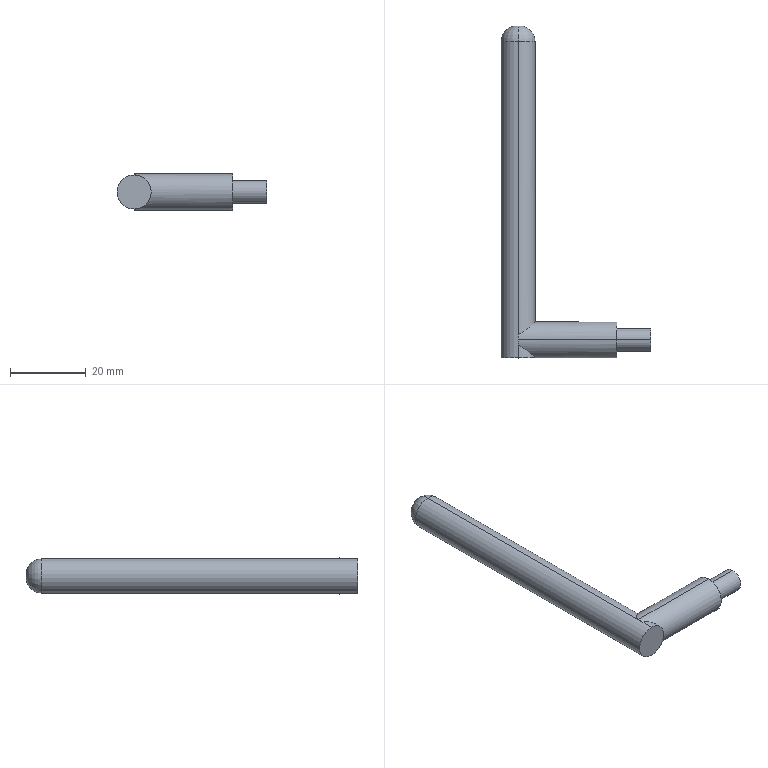Part | SolidWorks | features BaseBody 1 | 1 solid | 16 faces | box 39.5 x 87.5 x 9.5 mm | volume 7324 mm3 | cylinder 8 | plane 6 | torus 2 | commonest cylinder face diameters 9 x4 6 x2 9.5 x2
STEP:
#1=CARTESIAN_POINT('',(4.5,0.,0.));
#2=VERTEX_POINT('',#1);
#3=CARTESIAN_POINT('',(0.,0.,-4.5));
#4=VERTEX_POINT('',#3);
#5=CARTESIAN_POINT('',(0.,0.,0.));
#6=DIRECTION('',(0.,1.,0.));
#7=DIRECTION('',(0.,0.,1.));
#8=AXIS2_PLACEMENT_3D('',#5,#6,#7);
#9=CIRCLE('',#8,4.5);
#10=EDGE_CURVE('',#2,#4,#9,.T.);
#11=ORIENTED_EDGE('',*,*,#10,.T.);
#12=CARTESIAN_POINT('',(0.,3.229,-4.5));
#13=VERTEX_POINT('',#12);
#14=CARTESIAN_POINT('',(0.,0.,-4.5));
#15=DIRECTION('',(0.,1.,0.));
#16=VECTOR('',#15,1000.);
#17=LINE('',#14,#16);
#18=EDGE_CURVE('',#4,#13,#17,.T.);
#19=ORIENTED_EDGE('',*,*,#18,.T.);
#20=CARTESIAN_POINT('',(0.,3.229,-4.5));
#21=CARTESIAN_POINT('',(0.3352,3.229,-4.5));
#22=CARTESIAN_POINT('',(0.6529,3.113,-4.462));
#23=CARTESIAN_POINT('',(1.226,2.812,-4.34));
#24=CARTESIAN_POINT('',(1.491,2.627,-4.254));
#25=CARTESIAN_POINT('',(1.988,2.252,-4.046));
#26=CARTESIAN_POINT('',(2.223,2.06,-3.922));
#27=CARTESIAN_POINT('',(2.671,1.679,-3.632));
#28=CARTESIAN_POINT('',(2.886,1.489,-3.463));
#29=CARTESIAN_POINT('',(3.287,1.129,-3.085));
#30=CARTESIAN_POINT('',(3.473,0.9592,-2.876));
#31=CARTESIAN_POINT('',(3.813,0.6459,-2.408));
#32=CARTESIAN_POINT('',(3.966,0.5023,-2.147));
#33=CARTESIAN_POINT('',(4.157,0.3236,-1.73));
#34=CARTESIAN_POINT('',(4.214,0.2697,-1.586));
#35=CARTESIAN_POINT('',(4.315,0.1747,-1.286));
#36=CARTESIAN_POINT('',(4.359,0.1335,-1.13));
#37=CARTESIAN_POINT('',(4.463,0.03469,-0.6571));
#38=CARTESIAN_POINT('',(4.5,0.,-0.3334));
#39=CARTESIAN_POINT('',(4.5,0.,0.));
#40=B_SPLINE_CURVE_WITH_KNOTS('',3,(#20,#21,#22,#23,#24,#25,#26,#27,#28,#29,#30,#31,#32,#33,#34,#35,#36,#37,#38,#39),.UNSPECIFIED.,.F.,.F.,(4,2,2,2,2,2,2,2,2,4),(0.,0.0009882,0.001976,0.002964,0.003953,0.004941,0.005929,0.006423,0.006917,0.007905),.UNSPECIFIED.);
#41=EDGE_CURVE('',#13,#2,#40,.T.);
#42=ORIENTED_EDGE('',*,*,#41,.T.);
#43=EDGE_LOOP('',(#11,#19,#42));
#44=FACE_OUTER_BOUND('',#43,.T.);
#45=CARTESIAN_POINT('',(0.,0.,0.));
#46=DIRECTION('',(0.,1.,0.));
#47=DIRECTION('',(0.,0.,1.));
#48=AXIS2_PLACEMENT_3D('',#45,#46,#47);
#49=CYLINDRICAL_SURFACE('',#48,4.5);
#50=ADVANCED_FACE('',(#44),#49,.T.);
#51=CARTESIAN_POINT('',(0.,6.271,4.5));
#52=VERTEX_POINT('',#51);
#53=CARTESIAN_POINT('',(0.,6.271,-4.5));
#54=VERTEX_POINT('',#53);
#55=CARTESIAN_POINT('',(0.,6.271,4.5));
#56=CARTESIAN_POINT('',(0.3351,6.271,4.5));
#57=CARTESIAN_POINT('',(0.6528,6.387,4.462));
#58=CARTESIAN_POINT('',(1.226,6.688,4.34));
#59=CARTESIAN_POINT('',(1.491,6.873,4.254));
#60=CARTESIAN_POINT('',(1.988,7.248,4.046));
#61=CARTESIAN_POINT('',(2.222,7.44,3.922));
#62=CARTESIAN_POINT('',(2.671,7.821,3.632));
#63=CARTESIAN_POINT('',(2.886,8.011,3.464));
#64=CARTESIAN_POINT('',(3.287,8.371,3.086));
#65=CARTESIAN_POINT('',(3.473,8.541,2.876));
#66=CARTESIAN_POINT('',(3.812,8.854,2.408));
#67=CARTESIAN_POINT('',(3.966,8.997,2.148));
#68=CARTESIAN_POINT('',(4.157,9.176,1.731));
#69=CARTESIAN_POINT('',(4.214,9.23,1.586));
#70=CARTESIAN_POINT('',(4.315,9.325,1.287));
#71=CARTESIAN_POINT('',(4.359,9.366,1.13));
#72=CARTESIAN_POINT('',(4.463,9.465,0.6581));
#73=CARTESIAN_POINT('',(4.5,9.5,0.3345));
#74=CARTESIAN_POINT('',(4.5,9.5,-0.3323));
#75=CARTESIAN_POINT('',(4.464,9.465,-0.6563));
#76=CARTESIAN_POINT('',(4.359,9.367,-1.129));
#77=CARTESIAN_POINT('',(4.315,9.325,-1.286));
#78=CARTESIAN_POINT('',(4.214,9.23,-1.585));
#79=CARTESIAN_POINT('',(4.157,9.176,-1.73));
#80=CARTESIAN_POINT('',(3.966,8.997,-2.148));
#81=CARTESIAN_POINT('',(3.812,8.854,-2.409));
#82=CARTESIAN_POINT('',(3.473,8.541,-2.876));
#83=CARTESIAN_POINT('',(3.287,8.371,-3.086));
#84=CARTESIAN_POINT('',(2.885,8.01,-3.464));
#85=CARTESIAN_POINT('',(2.67,7.821,-3.632));
#86=CARTESIAN_POINT('',(2.223,7.441,-3.922));
#87=CARTESIAN_POINT('',(1.989,7.249,-4.045));
#88=CARTESIAN_POINT('',(1.492,6.874,-4.254));
#89=CARTESIAN_POINT('',(1.228,6.689,-4.339));
#90=CARTESIAN_POINT('',(0.7968,6.462,-4.431));
#91=CARTESIAN_POINT('',(0.6452,6.395,-4.456));
#92=CARTESIAN_POINT('',(0.3315,6.299,-4.491));
#93=CARTESIAN_POINT('',(0.1672,6.271,-4.5));
#94=CARTESIAN_POINT('',(0.,6.271,-4.5));
#95=B_SPLINE_CURVE_WITH_KNOTS('',3,(#55,#56,#57,#58,#59,#60,#61,#62,#63,#64,#65,#66,#67,#68,#69,#70,#71,#72,#73,#74,#75,#76,#77,#78,#79,#80,#81,#82,#83,#84,#85,#86,#87,#88,#89,#90,#91,#92,#93,#94),.UNSPECIFIED.,.F.,.F.,(4,2,2,2,2,2,2,2,2,2,2,2,2,2,2,2,2,2,2,4),(-0.007866,-0.006883,-0.005899,-0.004916,-0.003933,-0.00295,-0.001967,-0.001476,-0.0009841,-0.000001079,0.000982,0.001474,0.001965,0.002948,0.003931,0.004914,0.005897,0.00688,0.007372,0.007863),.UNSPECIFIED.);
#96=EDGE_CURVE('',#52,#54,#95,.T.);
#97=ORIENTED_EDGE('',*,*,#96,.T.);
#98=CARTESIAN_POINT('',(0.,83.5,-4.5));
#99=VERTEX_POINT('',#98);
#100=CARTESIAN_POINT('',(0.,0.,-4.5));
#101=DIRECTION('',(0.,1.,0.));
#102=VECTOR('',#101,1000.);
#103=LINE('',#100,#102);
#104=EDGE_CURVE('',#54,#99,#103,.T.);
#105=ORIENTED_EDGE('',*,*,#104,.T.);
#106=CARTESIAN_POINT('',(0.,83.5,4.5));
#107=VERTEX_POINT('',#106);
#108=CARTESIAN_POINT('',(0.,83.5,0.));
#109=DIRECTION('',(0.,-1.,0.));
#110=DIRECTION('',(0.,0.,1.));
#111=AXIS2_PLACEMENT_3D('',#108,#109,#110);
#112=CIRCLE('',#111,4.5);
#113=EDGE_CURVE('',#99,#107,#112,.T.);
#114=ORIENTED_EDGE('',*,*,#113,.T.);
#115=CARTESIAN_POINT('',(0.,0.,4.5));
#116=DIRECTION('',(0.,1.,0.));
#117=VECTOR('',#116,1000.);
#118=LINE('',#115,#117);
#119=EDGE_CURVE('',#52,#107,#118,.T.);
#120=ORIENTED_EDGE('',*,*,#119,.F.);
#121=EDGE_LOOP('',(#97,#105,#114,#120));
#122=FACE_OUTER_BOUND('',#121,.T.);
#123=CARTESIAN_POINT('',(0.,0.,0.));
#124=DIRECTION('',(0.,1.,0.));
#125=DIRECTION('',(0.,0.,1.));
#126=AXIS2_PLACEMENT_3D('',#123,#124,#125);
#127=CYLINDRICAL_SURFACE('',#126,4.5);
#128=ADVANCED_FACE('',(#122),#127,.T.);
#129=ORIENTED_EDGE('',*,*,#18,.F.);
#130=CARTESIAN_POINT('',(0.,0.,4.5));
#131=VERTEX_POINT('',#130);
#132=CARTESIAN_POINT('',(0.,0.,0.));
#133=DIRECTION('',(0.,1.,0.));
#134=DIRECTION('',(0.,0.,1.));
#135=AXIS2_PLACEMENT_3D('',#132,#133,#134);
#136=CIRCLE('',#135,4.5);
#137=EDGE_CURVE('',#4,#131,#136,.T.);
#138=ORIENTED_EDGE('',*,*,#137,.T.);
#139=CARTESIAN_POINT('',(0.,3.229,4.5));
#140=VERTEX_POINT('',#139);
#141=CARTESIAN_POINT('',(0.,0.,4.5));
#142=DIRECTION('',(0.,1.,0.));
#143=VECTOR('',#142,1000.);
#144=LINE('',#141,#143);
#145=EDGE_CURVE('',#131,#140,#144,.T.);
#146=ORIENTED_EDGE('',*,*,#145,.T.);
#147=CARTESIAN_POINT('',(0.,0.,4.5));
#148=DIRECTION('',(0.,1.,0.));
#149=VECTOR('',#148,1000.);
#150=LINE('',#147,#149);
#151=EDGE_CURVE('',#140,#52,#150,.T.);
#152=ORIENTED_EDGE('',*,*,#151,.T.);
#153=ORIENTED_EDGE('',*,*,#119,.T.);
#154=CARTESIAN_POINT('',(0.,83.5,0.));
#155=DIRECTION('',(0.,-1.,0.));
#156=DIRECTION('',(0.,0.,1.));
#157=AXIS2_PLACEMENT_3D('',#154,#155,#156);
#158=CIRCLE('',#157,4.5);
#159=EDGE_CURVE('',#107,#99,#158,.T.);
#160=ORIENTED_EDGE('',*,*,#159,.T.);
#161=ORIENTED_EDGE('',*,*,#104,.F.);
#162=CARTESIAN_POINT('',(0.,0.,-4.5));
#163=DIRECTION('',(0.,-1.,0.));
#164=VECTOR('',#163,1000.);
#165=LINE('',#162,#164);
#166=EDGE_CURVE('',#54,#13,#165,.T.);
#167=ORIENTED_EDGE('',*,*,#166,.T.);
#168=EDGE_LOOP('',(#129,#138,#146,#152,#153,#160,#161,#167));
#169=FACE_OUTER_BOUND('',#168,.T.);
#170=CARTESIAN_POINT('',(0.,0.,0.));
#171=DIRECTION('',(0.,1.,0.));
#172=DIRECTION('',(0.,0.,1.));
#173=AXIS2_PLACEMENT_3D('',#170,#171,#172);
#174=CYLINDRICAL_SURFACE('',#173,4.5);
#175=ADVANCED_FACE('',(#169),#174,.T.);
#176=ORIENTED_EDGE('',*,*,#113,.F.);
#177=CARTESIAN_POINT('',(0.,87.5,-0.5));
#178=VERTEX_POINT('',#177);
#179=CARTESIAN_POINT('',(0.,83.5,-0.5));
#180=DIRECTION('',(1.,0.,0.));
#181=DIRECTION('',(0.,0.,-1.));
#182=AXIS2_PLACEMENT_3D('',#179,#180,#181);
#183=CIRCLE('',#182,4.);
#184=EDGE_CURVE('',#99,#178,#183,.T.);
#185=ORIENTED_EDGE('',*,*,#184,.T.);
#186=CARTESIAN_POINT('',(0.,87.5,0.5));
#187=VERTEX_POINT('',#186);
#188=CARTESIAN_POINT('',(0.,87.5,0.));
#189=DIRECTION('',(0.,-1.,0.));
#190=DIRECTION('',(0.,0.,1.));
#191=AXIS2_PLACEMENT_3D('',#188,#189,#190);
#192=CIRCLE('',#191,0.5);
#193=EDGE_CURVE('',#178,#187,#192,.T.);
#194=ORIENTED_EDGE('',*,*,#193,.T.);
#195=CARTESIAN_POINT('',(0.,83.5,0.5));
#196=DIRECTION('',(-1.,0.,0.));
#197=DIRECTION('',(0.,0.,1.));
#198=AXIS2_PLACEMENT_3D('',#195,#196,#197);
#199=CIRCLE('',#198,4.);
#200=EDGE_CURVE('',#107,#187,#199,.T.);
#201=ORIENTED_EDGE('',*,*,#200,.F.);
#202=EDGE_LOOP('',(#176,#185,#194,#201));
#203=FACE_OUTER_BOUND('',#202,.T.);
#204=CARTESIAN_POINT('',(0.,83.5,0.));
#205=DIRECTION('',(0.,1.,0.));
#206=DIRECTION('',(0.,0.,1.));
#207=AXIS2_PLACEMENT_3D('',#204,#205,#206);
#208=TOROIDAL_SURFACE('',#207,0.5,4.);
#209=ADVANCED_FACE('',(#203),#208,.T.);
#210=CARTESIAN_POINT('',(0.,4.75,4.75));
#211=VERTEX_POINT('',#210);
#212=CARTESIAN_POINT('',(0.,4.75,0.));
#213=DIRECTION('',(1.,0.,0.));
#214=DIRECTION('',(0.,0.,-1.));
#215=AXIS2_PLACEMENT_3D('',#212,#213,#214);
#216=CIRCLE('',#215,4.75);
#217=EDGE_CURVE('',#52,#211,#216,.T.);
#218=ORIENTED_EDGE('',*,*,#217,.T.);
#219=CARTESIAN_POINT('',(26.,4.75,4.75));
#220=VERTEX_POINT('',#219);
#221=CARTESIAN_POINT('',(0.,4.75,4.75));
#222=DIRECTION('',(1.,0.,0.));
#223=VECTOR('',#222,1000.);
#224=LINE('',#221,#223);
#225=EDGE_CURVE('',#211,#220,#224,.T.);
#226=ORIENTED_EDGE('',*,*,#225,.T.);
#227=CARTESIAN_POINT('',(26.,4.75,-4.75));
#228=VERTEX_POINT('',#227);
#229=CARTESIAN_POINT('',(26.,4.75,0.));
#230=DIRECTION('',(-1.,0.,0.));
#231=DIRECTION('',(0.,0.,-1.));
#232=AXIS2_PLACEMENT_3D('',#229,#230,#231);
#233=CIRCLE('',#232,4.75);
#234=EDGE_CURVE('',#220,#228,#233,.T.);
#235=ORIENTED_EDGE('',*,*,#234,.T.);
#236=CARTESIAN_POINT('',(0.,4.75,-4.75));
#237=VERTEX_POINT('',#236);
#238=CARTESIAN_POINT('',(0.,4.75,-4.75));
#239=DIRECTION('',(1.,0.,0.));
#240=VECTOR('',#239,1000.);
#241=LINE('',#238,#240);
#242=EDGE_CURVE('',#237,#228,#241,.T.);
#243=ORIENTED_EDGE('',*,*,#242,.F.);
#244=CARTESIAN_POINT('',(0.,4.75,0.));
#245=DIRECTION('',(1.,0.,0.));
#246=DIRECTION('',(0.,0.,-1.));
#247=AXIS2_PLACEMENT_3D('',#244,#245,#246);
#248=CIRCLE('',#247,4.75);
#249=EDGE_CURVE('',#237,#54,#248,.T.);
#250=ORIENTED_EDGE('',*,*,#249,.T.);
#251=ORIENTED_EDGE('',*,*,#96,.F.);
#252=EDGE_LOOP('',(#218,#226,#235,#243,#250,#251));
#253=FACE_OUTER_BOUND('',#252,.T.);
#254=CARTESIAN_POINT('',(0.,4.75,0.));
#255=DIRECTION('',(1.,0.,0.));
#256=DIRECTION('',(0.,0.,-1.));
#257=AXIS2_PLACEMENT_3D('',#254,#255,#256);
#258=CYLINDRICAL_SURFACE('',#257,4.75);
#259=ADVANCED_FACE('',(#253),#258,.T.);
#260=CARTESIAN_POINT('',(26.,4.75,3.));
#261=VERTEX_POINT('',#260);
#262=CARTESIAN_POINT('',(26.,4.75,-3.));
#263=VERTEX_POINT('',#262);
#264=CARTESIAN_POINT('',(26.,4.75,0.));
#265=DIRECTION('',(-1.,0.,0.));
#266=DIRECTION('',(0.,0.,-1.));
#267=AXIS2_PLACEMENT_3D('',#264,#265,#266);
#268=CIRCLE('',#267,3.);
#269=EDGE_CURVE('',#261,#263,#268,.T.);
#270=ORIENTED_EDGE('',*,*,#269,.F.);
#271=CARTESIAN_POINT('',(35.,4.75,3.));
#272=VERTEX_POINT('',#271);
#273=CARTESIAN_POINT('',(35.,4.75,3.));
#274=DIRECTION('',(1.,0.,0.));
#275=VECTOR('',#274,1000.);
#276=LINE('',#273,#275);
#277=EDGE_CURVE('',#261,#272,#276,.T.);
#278=ORIENTED_EDGE('',*,*,#277,.T.);
#279=CARTESIAN_POINT('',(35.,4.75,-3.));
#280=VERTEX_POINT('',#279);
#281=CARTESIAN_POINT('',(35.,4.75,0.));
#282=DIRECTION('',(-1.,0.,0.));
#283=DIRECTION('',(0.,0.,-1.));
#284=AXIS2_PLACEMENT_3D('',#281,#282,#283);
#285=CIRCLE('',#284,3.);
#286=EDGE_CURVE('',#272,#280,#285,.T.);
#287=ORIENTED_EDGE('',*,*,#286,.T.);
#288=CARTESIAN_POINT('',(35.,4.75,-3.));
#289=DIRECTION('',(1.,0.,0.));
#290=VECTOR('',#289,1000.);
#291=LINE('',#288,#290);
#292=EDGE_CURVE('',#263,#280,#291,.T.);
#293=ORIENTED_EDGE('',*,*,#292,.F.);
#294=EDGE_LOOP('',(#270,#278,#287,#293));
#295=FACE_OUTER_BOUND('',#294,.T.);
#296=CARTESIAN_POINT('',(35.,4.75,0.));
#297=DIRECTION('',(1.,0.,0.));
#298=DIRECTION('',(0.,0.,-1.));
#299=AXIS2_PLACEMENT_3D('',#296,#297,#298);
#300=CYLINDRICAL_SURFACE('',#299,3.);
#301=ADVANCED_FACE('',(#295),#300,.T.);
#302=ORIENTED_EDGE('',*,*,#145,.F.);
#303=CARTESIAN_POINT('',(0.,0.,0.));
#304=DIRECTION('',(0.,1.,0.));
#305=DIRECTION('',(0.,0.,1.));
#306=AXIS2_PLACEMENT_3D('',#303,#304,#305);
#307=CIRCLE('',#306,4.5);
#308=EDGE_CURVE('',#131,#2,#307,.T.);
#309=ORIENTED_EDGE('',*,*,#308,.T.);
#310=CARTESIAN_POINT('',(4.5,0.,0.));
#311=CARTESIAN_POINT('',(4.5,0.,0.3333));
#312=CARTESIAN_POINT('',(4.463,0.03467,0.6572));
#313=CARTESIAN_POINT('',(4.359,0.1336,1.13));
#314=CARTESIAN_POINT('',(4.315,0.1749,1.287));
#315=CARTESIAN_POINT('',(4.214,0.2699,1.586));
#316=CARTESIAN_POINT('',(4.157,0.3238,1.731));
#317=CARTESIAN_POINT('',(3.966,0.503,2.149));
#318=CARTESIAN_POINT('',(3.812,0.6468,2.409));
#319=CARTESIAN_POINT('',(3.473,0.9595,2.876));
#320=CARTESIAN_POINT('',(3.287,1.13,3.086));
#321=CARTESIAN_POINT('',(2.885,1.49,3.465));
#322=CARTESIAN_POINT('',(2.67,1.68,3.632));
#323=CARTESIAN_POINT('',(2.223,2.059,3.922));
#324=CARTESIAN_POINT('',(1.989,2.251,4.045));
#325=CARTESIAN_POINT('',(1.492,2.626,4.254));
#326=CARTESIAN_POINT('',(1.227,2.811,4.339));
#327=CARTESIAN_POINT('',(0.7967,3.038,4.431));
#328=CARTESIAN_POINT('',(0.6451,3.105,4.456));
#329=CARTESIAN_POINT('',(0.3315,3.201,4.491));
#330=CARTESIAN_POINT('',(0.1672,3.229,4.5));
#331=CARTESIAN_POINT('',(0.,3.229,4.5));
#332=B_SPLINE_CURVE_WITH_KNOTS('',3,(#310,#311,#312,#313,#314,#315,#316,#317,#318,#319,#320,#321,#322,#323,#324,#325,#326,#327,#328,#329,#330,#331),.UNSPECIFIED.,.F.,.F.,(4,2,2,2,2,2,2,2,2,2,4),(0.,0.0009829,0.001474,0.001966,0.002949,0.003932,0.004915,0.005898,0.006881,0.007372,0.007863),.UNSPECIFIED.);
#333=EDGE_CURVE('',#2,#140,#332,.T.);
#334=ORIENTED_EDGE('',*,*,#333,.T.);
#335=EDGE_LOOP('',(#302,#309,#334));
#336=FACE_OUTER_BOUND('',#335,.T.);
#337=CARTESIAN_POINT('',(0.,0.,0.));
#338=DIRECTION('',(0.,1.,0.));
#339=DIRECTION('',(0.,0.,1.));
#340=AXIS2_PLACEMENT_3D('',#337,#338,#339);
#341=CYLINDRICAL_SURFACE('',#340,4.5);
#342=ADVANCED_FACE('',(#336),#341,.T.);
#343=ORIENTED_EDGE('',*,*,#184,.F.);
#344=ORIENTED_EDGE('',*,*,#159,.F.);
#345=ORIENTED_EDGE('',*,*,#200,.T.);
#346=CARTESIAN_POINT('',(0.,87.5,0.));
#347=DIRECTION('',(0.,-1.,0.));
#348=DIRECTION('',(0.,0.,1.));
#349=AXIS2_PLACEMENT_3D('',#346,#347,#348);
#350=CIRCLE('',#349,0.5);
#351=EDGE_CURVE('',#187,#178,#350,.T.);
#352=ORIENTED_EDGE('',*,*,#351,.T.);
#353=EDGE_LOOP('',(#343,#344,#345,#352));
#354=FACE_OUTER_BOUND('',#353,.T.);
#355=CARTESIAN_POINT('',(0.,83.5,0.));
#356=DIRECTION('',(0.,1.,0.));
#357=DIRECTION('',(0.,0.,1.));
#358=AXIS2_PLACEMENT_3D('',#355,#356,#357);
#359=TOROIDAL_SURFACE('',#358,0.5,4.);
#360=ADVANCED_FACE('',(#354),#359,.T.);
#361=ORIENTED_EDGE('',*,*,#10,.F.);
#362=ORIENTED_EDGE('',*,*,#308,.F.);
#363=ORIENTED_EDGE('',*,*,#137,.F.);
#364=EDGE_LOOP('',(#361,#362,#363));
#365=FACE_OUTER_BOUND('',#364,.T.);
#366=CARTESIAN_POINT('',(0.,0.,0.));
#367=DIRECTION('',(0.,1.,0.));
#368=DIRECTION('',(0.,0.,1.));
#369=AXIS2_PLACEMENT_3D('',#366,#367,#368);
#370=PLANE('',#369);
#371=ADVANCED_FACE('',(#365),#370,.F.);
#372=ORIENTED_EDGE('',*,*,#225,.F.);
#373=CARTESIAN_POINT('',(0.,4.75,0.));
#374=DIRECTION('',(1.,0.,0.));
#375=DIRECTION('',(0.,0.,-1.));
#376=AXIS2_PLACEMENT_3D('',#373,#374,#375);
#377=CIRCLE('',#376,4.75);
#378=EDGE_CURVE('',#211,#140,#377,.T.);
#379=ORIENTED_EDGE('',*,*,#378,.T.);
#380=ORIENTED_EDGE('',*,*,#333,.F.);
#381=ORIENTED_EDGE('',*,*,#41,.F.);
#382=CARTESIAN_POINT('',(0.,4.75,0.));
#383=DIRECTION('',(1.,0.,0.));
#384=DIRECTION('',(0.,0.,-1.));
#385=AXIS2_PLACEMENT_3D('',#382,#383,#384);
#386=CIRCLE('',#385,4.75);
#387=EDGE_CURVE('',#13,#237,#386,.T.);
#388=ORIENTED_EDGE('',*,*,#387,.T.);
#389=ORIENTED_EDGE('',*,*,#242,.T.);
#390=CARTESIAN_POINT('',(26.,4.75,0.));
#391=DIRECTION('',(-1.,0.,0.));
#392=DIRECTION('',(0.,0.,-1.));
#393=AXIS2_PLACEMENT_3D('',#390,#391,#392);
#394=CIRCLE('',#393,4.75);
#395=EDGE_CURVE('',#228,#220,#394,.T.);
#396=ORIENTED_EDGE('',*,*,#395,.T.);
#397=EDGE_LOOP('',(#372,#379,#380,#381,#388,#389,#396));
#398=FACE_OUTER_BOUND('',#397,.T.);
#399=CARTESIAN_POINT('',(0.,4.75,0.));
#400=DIRECTION('',(1.,0.,0.));
#401=DIRECTION('',(0.,0.,-1.));
#402=AXIS2_PLACEMENT_3D('',#399,#400,#401);
#403=CYLINDRICAL_SURFACE('',#402,4.75);
#404=ADVANCED_FACE('',(#398),#403,.T.);
#405=ORIENTED_EDGE('',*,*,#166,.F.);
#406=ORIENTED_EDGE('',*,*,#249,.F.);
#407=ORIENTED_EDGE('',*,*,#387,.F.);
#408=EDGE_LOOP('',(#405,#406,#407));
#409=FACE_OUTER_BOUND('',#408,.T.);
#410=CARTESIAN_POINT('',(0.,0.,0.));
#411=DIRECTION('',(1.,0.,0.));
#412=DIRECTION('',(0.,0.,-1.));
#413=AXIS2_PLACEMENT_3D('',#410,#411,#412);
#414=PLANE('',#413);
#415=ADVANCED_FACE('',(#409),#414,.F.);
#416=ORIENTED_EDGE('',*,*,#351,.F.);
#417=ORIENTED_EDGE('',*,*,#193,.F.);
#418=EDGE_LOOP('',(#416,#417));
#419=FACE_OUTER_BOUND('',#418,.T.);
#420=CARTESIAN_POINT('',(0.,87.5,0.));
#421=DIRECTION('',(0.,1.,0.));
#422=DIRECTION('',(0.,0.,1.));
#423=AXIS2_PLACEMENT_3D('',#420,#421,#422);
#424=PLANE('',#423);
#425=ADVANCED_FACE('',(#419),#424,.T.);
#426=ORIENTED_EDGE('',*,*,#151,.F.);
#427=ORIENTED_EDGE('',*,*,#378,.F.);
#428=ORIENTED_EDGE('',*,*,#217,.F.);
#429=EDGE_LOOP('',(#426,#427,#428));
#430=FACE_OUTER_BOUND('',#429,.T.);
#431=CARTESIAN_POINT('',(0.,0.,0.));
#432=DIRECTION('',(1.,0.,0.));
#433=DIRECTION('',(0.,0.,-1.));
#434=AXIS2_PLACEMENT_3D('',#431,#432,#433);
#435=PLANE('',#434);
#436=ADVANCED_FACE('',(#430),#435,.F.);
#437=CARTESIAN_POINT('',(26.,4.75,0.));
#438=DIRECTION('',(-1.,0.,0.));
#439=DIRECTION('',(0.,0.,-1.));
#440=AXIS2_PLACEMENT_3D('',#437,#438,#439);
#441=CIRCLE('',#440,3.);
#442=EDGE_CURVE('',#263,#261,#441,.T.);
#443=ORIENTED_EDGE('',*,*,#442,.T.);
#444=ORIENTED_EDGE('',*,*,#269,.T.);
#445=EDGE_LOOP('',(#443,#444));
#446=FACE_BOUND('',#445,.T.);
#447=ORIENTED_EDGE('',*,*,#395,.F.);
#448=ORIENTED_EDGE('',*,*,#234,.F.);
#449=EDGE_LOOP('',(#447,#448));
#450=FACE_OUTER_BOUND('',#449,.T.);
#451=CARTESIAN_POINT('',(26.,0.,0.));
#452=DIRECTION('',(1.,0.,0.));
#453=DIRECTION('',(0.,0.,-1.));
#454=AXIS2_PLACEMENT_3D('',#451,#452,#453);
#455=PLANE('',#454);
#456=ADVANCED_FACE('',(#446,#450),#455,.T.);
#457=ORIENTED_EDGE('',*,*,#277,.F.);
#458=ORIENTED_EDGE('',*,*,#442,.F.);
#459=ORIENTED_EDGE('',*,*,#292,.T.);
#460=CARTESIAN_POINT('',(35.,4.75,0.));
#461=DIRECTION('',(-1.,0.,0.));
#462=DIRECTION('',(0.,0.,-1.));
#463=AXIS2_PLACEMENT_3D('',#460,#461,#462);
#464=CIRCLE('',#463,3.);
#465=EDGE_CURVE('',#280,#272,#464,.T.);
#466=ORIENTED_EDGE('',*,*,#465,.T.);
#467=EDGE_LOOP('',(#457,#458,#459,#466));
#468=FACE_OUTER_BOUND('',#467,.T.);
#469=CARTESIAN_POINT('',(35.,4.75,0.));
#470=DIRECTION('',(1.,0.,0.));
#471=DIRECTION('',(0.,0.,-1.));
#472=AXIS2_PLACEMENT_3D('',#469,#470,#471);
#473=CYLINDRICAL_SURFACE('',#472,3.);
#474=ADVANCED_FACE('',(#468),#473,.T.);
#475=ORIENTED_EDGE('',*,*,#465,.F.);
#476=ORIENTED_EDGE('',*,*,#286,.F.);
#477=EDGE_LOOP('',(#475,#476));
#478=FACE_OUTER_BOUND('',#477,.T.);
#479=CARTESIAN_POINT('',(35.,0.,0.));
#480=DIRECTION('',(1.,0.,0.));
#481=DIRECTION('',(0.,0.,-1.));
#482=AXIS2_PLACEMENT_3D('',#479,#480,#481);
#483=PLANE('',#482);
#484=ADVANCED_FACE('',(#478),#483,.T.);
#485=CLOSED_SHELL('',(#50,#128,#175,#209,#259,#301,#342,#360,#371,#404,#415,#425,#436,#456,#474,#484));
#486=MANIFOLD_SOLID_BREP('',#485);
#487=CARTESIAN_POINT('',(0.,0.,0.));
#488=DIRECTION('',(0.,0.,1.));
#489=DIRECTION('',(1.,0.,0.));
#490=AXIS2_PLACEMENT_3D('',#487,#488,#489);
#491=(LENGTH_UNIT()NAMED_UNIT(*)SI_UNIT(.MILLI.,.METRE.));
#492=UNCERTAINTY_MEASURE_WITH_UNIT(LENGTH_MEASURE(0.00001),#491,'','');
#493=(NAMED_UNIT(*)PLANE_ANGLE_UNIT()SI_UNIT($,.RADIAN.));
#494=(NAMED_UNIT(*)SI_UNIT($,.STERADIAN.)SOLID_ANGLE_UNIT());
#495=(GEOMETRIC_REPRESENTATION_CONTEXT(3)GLOBAL_UNCERTAINTY_ASSIGNED_CONTEXT((#492))GLOBAL_UNIT_ASSIGNED_CONTEXT((#491,#493,#494))REPRESENTATION_CONTEXT('',''));
#496=ADVANCED_BREP_SHAPE_REPRESENTATION('',(#486,#490),#495);